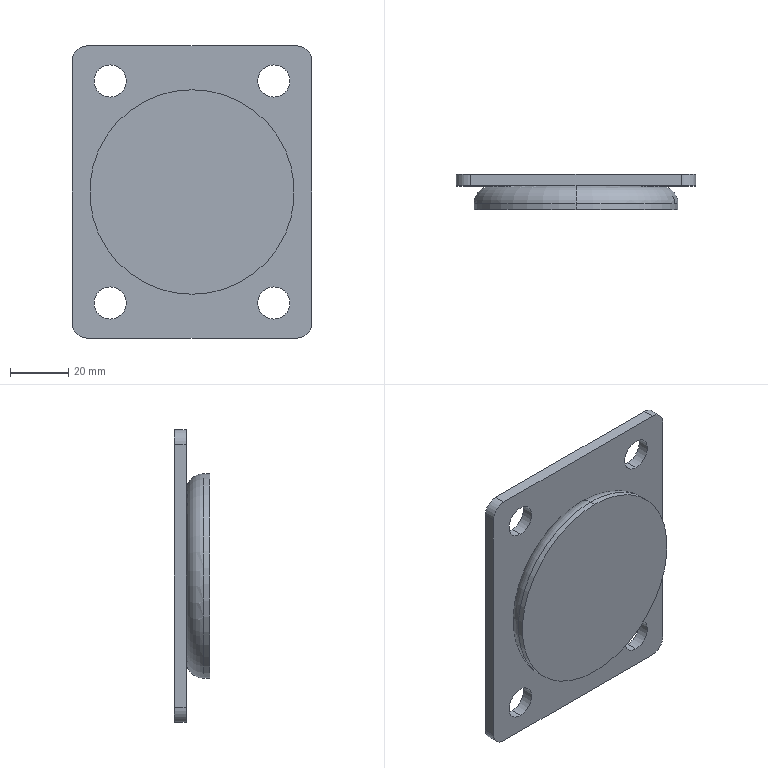Part | SolidWorks | features BaseBody 1 | 1 solid | 26 faces | box 82 x 12 x 100 mm | volume 48810 mm3 | cylinder 16 | plane 8 | torus 2 | commonest cylinder face diameters 11 x8 10 x4 70 x4
STEP:
#1=CARTESIAN_POINT('',(0.,60.5,21.));
#2=VERTEX_POINT('',#1);
#3=CARTESIAN_POINT('',(0.,60.5,-49.));
#4=VERTEX_POINT('',#3);
#5=CARTESIAN_POINT('',(0.,60.5,-14.));
#6=DIRECTION('',(0.,1.,0.));
#7=DIRECTION('',(0.,0.,1.));
#8=AXIS2_PLACEMENT_3D('',#5,#6,#7);
#9=CIRCLE('',#8,35.);
#10=EDGE_CURVE('',#2,#4,#9,.T.);
#11=ORIENTED_EDGE('',*,*,#10,.T.);
#12=CARTESIAN_POINT('',(0.,66.5,-43.));
#13=VERTEX_POINT('',#12);
#14=CARTESIAN_POINT('',(0.,60.5,-43.));
#15=DIRECTION('',(1.,0.,0.));
#16=DIRECTION('',(0.,0.,-1.));
#17=AXIS2_PLACEMENT_3D('',#14,#15,#16);
#18=CIRCLE('',#17,6.);
#19=EDGE_CURVE('',#4,#13,#18,.T.);
#20=ORIENTED_EDGE('',*,*,#19,.T.);
#21=CARTESIAN_POINT('',(0.,66.5,15.));
#22=VERTEX_POINT('',#21);
#23=CARTESIAN_POINT('',(0.,66.5,-43.));
#24=CARTESIAN_POINT('',(1.148,66.5,-43.));
#25=CARTESIAN_POINT('',(2.232,66.5,-42.932));
#26=CARTESIAN_POINT('',(4.262,66.5,-42.703));
#27=CARTESIAN_POINT('',(5.208,66.5,-42.542));
#28=CARTESIAN_POINT('',(7.832,66.5,-41.979));
#29=CARTESIAN_POINT('',(9.297,66.5,-41.499));
#30=CARTESIAN_POINT('',(11.688,66.5,-40.571));
#31=CARTESIAN_POINT('',(12.616,66.5,-40.124));
#32=CARTESIAN_POINT('',(13.391,66.5,-39.723));
#33=CARTESIAN_POINT('',(13.515,66.5,-39.659));
#34=CARTESIAN_POINT('',(13.635,66.5,-39.595));
#35=CARTESIAN_POINT('',(13.679,66.5,-39.571));
#36=CARTESIAN_POINT('',(13.686,66.5,-39.568));
#37=CARTESIAN_POINT('',(13.691,66.5,-39.565));
#38=CARTESIAN_POINT('',(13.699,66.5,-39.561));
#39=CARTESIAN_POINT('',(13.732,66.5,-39.543));
#40=CARTESIAN_POINT('',(13.81,66.5,-39.501));
#41=CARTESIAN_POINT('',(14.304,66.5,-39.232));
#42=CARTESIAN_POINT('',(14.766,66.5,-38.964));
#43=CARTESIAN_POINT('',(15.982,66.5,-38.218));
#44=CARTESIAN_POINT('',(16.772,66.5,-37.678));
#45=CARTESIAN_POINT('',(18.3,66.5,-36.518));
#46=CARTESIAN_POINT('',(19.038,66.5,-35.898));
#47=CARTESIAN_POINT('',(19.836,66.5,-35.156));
#48=CARTESIAN_POINT('',(19.924,66.5,-35.073));
#49=CARTESIAN_POINT('',(20.033,66.5,-34.969));
#50=CARTESIAN_POINT('',(20.056,66.5,-34.947));
#51=CARTESIAN_POINT('',(20.104,66.5,-34.901));
#52=CARTESIAN_POINT('',(20.175,66.5,-34.832));
#53=CARTESIAN_POINT('',(20.438,66.5,-34.577));
#54=CARTESIAN_POINT('',(21.047,66.5,-33.964));
#55=CARTESIAN_POINT('',(21.585,66.5,-33.374));
#56=CARTESIAN_POINT('',(22.63,66.5,-32.167));
#57=CARTESIAN_POINT('',(23.281,66.5,-31.324));
#58=CARTESIAN_POINT('',(24.036,66.5,-30.229));
#59=CARTESIAN_POINT('',(24.182,66.5,-30.011));
#60=CARTESIAN_POINT('',(24.481,66.5,-29.549));
#61=CARTESIAN_POINT('',(24.774,66.5,-29.084));
#62=CARTESIAN_POINT('',(25.123,66.5,-28.491));
#63=CARTESIAN_POINT('',(25.329,66.5,-28.124));
#64=CARTESIAN_POINT('',(25.399,66.5,-27.996));
#65=CARTESIAN_POINT('',(25.405,66.5,-27.985));
#66=CARTESIAN_POINT('',(25.408,66.5,-27.98));
#67=CARTESIAN_POINT('',(25.409,66.5,-27.978));
#68=CARTESIAN_POINT('',(25.411,66.5,-27.974));
#69=CARTESIAN_POINT('',(25.418,66.5,-27.962));
#70=CARTESIAN_POINT('',(25.435,66.5,-27.93));
#71=CARTESIAN_POINT('',(25.456,66.5,-27.892));
#72=CARTESIAN_POINT('',(25.538,66.5,-27.742));
#73=CARTESIAN_POINT('',(25.642,66.5,-27.549));
#74=CARTESIAN_POINT('',(25.92,66.5,-27.009));
#75=CARTESIAN_POINT('',(26.094,66.5,-26.663));
#76=CARTESIAN_POINT('',(26.342,66.5,-26.129));
#77=CARTESIAN_POINT('',(26.394,66.5,-26.017));
#78=CARTESIAN_POINT('',(26.453,66.5,-25.886));
#79=CARTESIAN_POINT('',(26.46,66.5,-25.871));
#80=CARTESIAN_POINT('',(26.469,66.5,-25.849));
#81=CARTESIAN_POINT('',(26.471,66.5,-25.846));
#82=CARTESIAN_POINT('',(26.474,66.5,-25.839));
#83=CARTESIAN_POINT('',(26.482,66.5,-25.821));
#84=CARTESIAN_POINT('',(26.503,66.5,-25.774));
#85=CARTESIAN_POINT('',(26.573,66.5,-25.615));
#86=CARTESIAN_POINT('',(26.638,66.5,-25.466));
#87=CARTESIAN_POINT('',(26.793,66.5,-25.101));
#88=CARTESIAN_POINT('',(26.897,66.5,-24.848));
#89=CARTESIAN_POINT('',(27.208,66.5,-24.054));
#90=CARTESIAN_POINT('',(27.415,66.5,-23.481));
#91=CARTESIAN_POINT('',(27.637,66.5,-22.788));
#92=CARTESIAN_POINT('',(27.674,66.5,-22.671));
#93=CARTESIAN_POINT('',(27.711,66.5,-22.553));
#94=CARTESIAN_POINT('',(27.726,66.5,-22.503));
#95=CARTESIAN_POINT('',(27.73,66.5,-22.49));
#96=CARTESIAN_POINT('',(27.731,66.5,-22.485));
#97=CARTESIAN_POINT('',(27.734,66.5,-22.477));
#98=CARTESIAN_POINT('',(27.75,66.5,-22.424));
#99=CARTESIAN_POINT('',(27.767,66.5,-22.367));
#100=CARTESIAN_POINT('',(27.817,66.5,-22.2));
#101=CARTESIAN_POINT('',(27.856,66.5,-22.068));
#102=CARTESIAN_POINT('',(27.987,66.5,-21.606));
#103=CARTESIAN_POINT('',(28.093,66.5,-21.214));
#104=CARTESIAN_POINT('',(28.322,66.5,-20.253));
#105=CARTESIAN_POINT('',(28.445,66.5,-19.685));
#106=CARTESIAN_POINT('',(28.677,66.5,-18.37));
#107=CARTESIAN_POINT('',(28.785,66.5,-17.622));
#108=CARTESIAN_POINT('',(28.906,66.5,-16.364));
#109=CARTESIAN_POINT('',(28.94,66.5,-15.923));
#110=CARTESIAN_POINT('',(28.975,66.5,-15.227));
#111=CARTESIAN_POINT('',(28.984,66.5,-14.989));
#112=CARTESIAN_POINT('',(28.994,66.5,-14.624));
#113=CARTESIAN_POINT('',(28.997,66.5,-14.44));
#114=CARTESIAN_POINT('',(28.999,66.5,-14.221));
#115=CARTESIAN_POINT('',(29.,66.5,-14.111));
#116=CARTESIAN_POINT('',(29.,66.5,-14.056));
#117=CARTESIAN_POINT('',(29.,66.5,-14.028));
#118=CARTESIAN_POINT('',(29.,66.5,-14.016));
#119=CARTESIAN_POINT('',(29.,66.5,-14.008));
#120=CARTESIAN_POINT('',(29.,66.5,-14.002));
#121=CARTESIAN_POINT('',(29.,66.5,-12.102));
#122=CARTESIAN_POINT('',(28.813,66.5,-10.204));
#123=CARTESIAN_POINT('',(28.073,66.5,-6.481));
#124=CARTESIAN_POINT('',(27.519,66.5,-4.656));
#125=CARTESIAN_POINT('',(26.066,66.5,-1.149));
#126=CARTESIAN_POINT('',(25.167,66.5,0.5335));
#127=CARTESIAN_POINT('',(23.058,66.5,3.69));
#128=CARTESIAN_POINT('',(21.848,66.5,5.164));
#129=CARTESIAN_POINT('',(19.164,66.5,7.848));
#130=CARTESIAN_POINT('',(17.69,66.5,9.058));
#131=CARTESIAN_POINT('',(14.533,66.5,11.167));
#132=CARTESIAN_POINT('',(12.851,66.5,12.066));
#133=CARTESIAN_POINT('',(9.344,66.5,13.519));
#134=CARTESIAN_POINT('',(7.519,66.5,14.073));
#135=CARTESIAN_POINT('',(3.796,66.5,14.813));
#136=CARTESIAN_POINT('',(1.898,66.5,15.));
#137=CARTESIAN_POINT('',(0.,66.5,15.));
#138=B_SPLINE_CURVE_WITH_KNOTS('',3,(#23,#24,#25,#26,#27,#28,#29,#30,#31,#32,#33,#34,#35,#36,#37,#38,#39,#40,#41,#42,#43,#44,#45,#46,#47,#48,#49,#50,#51,#52,#53,#54,#55,#56,#57,#58,#59,#60,#61,#62,#63,#64,#65,#66,#67,#68,#69,#70,#71,#72,#73,#74,#75,#76,#77,#78,#79,#80,#81,#82,#83,#84,#85,#86,#87,#88,#89,#90,#91,#92,#93,#94,#95,#96,#97,#98,#99,#100,#101,#102,#103,#104,#105,#106,#107,#108,#109,#110,#111,#112,#113,#114,#115,#116,#117,#118,#119,#120,#121,#122,#123,#124,#125,#126,#127,#128,#129,#130,#131,#132,#133,#134,#135,#136,#137),.UNSPECIFIED.,.F.,.F.,(4,2,2,2,2,1,1,1,2,2,1,1,2,2,2,2,2,1,1,1,2,2,2,1,1,1,2,2,1,1,1,2,2,2,2,2,2,1,1,1,2,2,2,1,2,2,1,1,2,2,2,2,2,2,2,1,1,1,1,1,2,2,2,2,2,2,2,2,2,4),(0.,0.03125,0.0625,0.125,0.1875,0.1953,0.1992,0.1997,0.2,0.2002,0.2012,0.2031,0.2188,0.25,0.2813,0.2852,0.2861,0.2871,0.2891,0.2969,0.3125,0.3438,0.3516,0.3594,0.3672,0.3711,0.3713,0.3715,0.3716,0.3721,0.373,0.375,0.3828,0.3906,0.3926,0.3928,0.3929,0.3931,0.3936,0.3945,0.3984,0.4063,0.4219,0.4238,0.4248,0.425,0.4253,0.4258,0.4297,0.4375,0.4531,0.4688,0.4844,0.4922,0.4961,0.498,0.499,0.4995,0.4998,0.4999,0.4999,0.5,0.5625,0.625,0.6875,0.75,0.8125,0.875,0.9375,1.),.UNSPECIFIED.);
#139=EDGE_CURVE('',#13,#22,#138,.T.);
#140=ORIENTED_EDGE('',*,*,#139,.T.);
#141=CARTESIAN_POINT('',(0.,60.5,15.));
#142=DIRECTION('',(-1.,0.,0.));
#143=DIRECTION('',(0.,0.,1.));
#144=AXIS2_PLACEMENT_3D('',#141,#142,#143);
#145=CIRCLE('',#144,6.);
#146=EDGE_CURVE('',#2,#22,#145,.T.);
#147=ORIENTED_EDGE('',*,*,#146,.F.);
#148=EDGE_LOOP('',(#11,#20,#140,#147));
#149=FACE_OUTER_BOUND('',#148,.T.);
#150=CARTESIAN_POINT('',(0.,60.5,-14.));
#151=DIRECTION('',(0.,1.,0.));
#152=DIRECTION('',(0.,0.,1.));
#153=AXIS2_PLACEMENT_3D('',#150,#151,#152);
#154=TOROIDAL_SURFACE('',#153,29.,6.);
#155=ADVANCED_FACE('',(#149),#154,.T.);
#156=CARTESIAN_POINT('',(-28.,66.5,-46.5));
#157=VERTEX_POINT('',#156);
#158=CARTESIAN_POINT('',(-28.,66.5,-57.5));
#159=VERTEX_POINT('',#158);
#160=CARTESIAN_POINT('',(-28.,66.5,-52.));
#161=DIRECTION('',(0.,-1.,0.));
#162=DIRECTION('',(0.,0.,1.));
#163=AXIS2_PLACEMENT_3D('',#160,#161,#162);
#164=CIRCLE('',#163,5.5);
#165=EDGE_CURVE('',#157,#159,#164,.T.);
#166=ORIENTED_EDGE('',*,*,#165,.T.);
#167=CARTESIAN_POINT('',(-28.,70.5,-57.5));
#168=VERTEX_POINT('',#167);
#169=CARTESIAN_POINT('',(-28.,58.5,-57.5));
#170=DIRECTION('',(0.,1.,0.));
#171=VECTOR('',#170,1000.);
#172=LINE('',#169,#171);
#173=EDGE_CURVE('',#159,#168,#172,.T.);
#174=ORIENTED_EDGE('',*,*,#173,.T.);
#175=CARTESIAN_POINT('',(-28.,70.5,-46.5));
#176=VERTEX_POINT('',#175);
#177=CARTESIAN_POINT('',(-28.,70.5,-52.));
#178=DIRECTION('',(0.,-1.,0.));
#179=DIRECTION('',(0.,0.,1.));
#180=AXIS2_PLACEMENT_3D('',#177,#178,#179);
#181=CIRCLE('',#180,5.5);
#182=EDGE_CURVE('',#176,#168,#181,.T.);
#183=ORIENTED_EDGE('',*,*,#182,.F.);
#184=CARTESIAN_POINT('',(-28.,58.5,-46.5));
#185=DIRECTION('',(0.,1.,0.));
#186=VECTOR('',#185,1000.);
#187=LINE('',#184,#186);
#188=EDGE_CURVE('',#157,#176,#187,.T.);
#189=ORIENTED_EDGE('',*,*,#188,.F.);
#190=EDGE_LOOP('',(#166,#174,#183,#189));
#191=FACE_OUTER_BOUND('',#190,.T.);
#192=CARTESIAN_POINT('',(-28.,58.5,-52.));
#193=DIRECTION('',(0.,1.,0.));
#194=DIRECTION('',(0.,0.,1.));
#195=AXIS2_PLACEMENT_3D('',#192,#193,#194);
#196=CYLINDRICAL_SURFACE('',#195,5.5);
#197=ADVANCED_FACE('',(#191),#196,.F.);
#198=CARTESIAN_POINT('',(28.,66.5,-46.5));
#199=VERTEX_POINT('',#198);
#200=CARTESIAN_POINT('',(28.,66.5,-57.5));
#201=VERTEX_POINT('',#200);
#202=CARTESIAN_POINT('',(28.,66.5,-52.));
#203=DIRECTION('',(0.,-1.,0.));
#204=DIRECTION('',(0.,0.,1.));
#205=AXIS2_PLACEMENT_3D('',#202,#203,#204);
#206=CIRCLE('',#205,5.5);
#207=EDGE_CURVE('',#199,#201,#206,.T.);
#208=ORIENTED_EDGE('',*,*,#207,.T.);
#209=CARTESIAN_POINT('',(28.,70.5,-57.5));
#210=VERTEX_POINT('',#209);
#211=CARTESIAN_POINT('',(28.,58.5,-57.5));
#212=DIRECTION('',(0.,1.,0.));
#213=VECTOR('',#212,1000.);
#214=LINE('',#211,#213);
#215=EDGE_CURVE('',#201,#210,#214,.T.);
#216=ORIENTED_EDGE('',*,*,#215,.T.);
#217=CARTESIAN_POINT('',(28.,70.5,-46.5));
#218=VERTEX_POINT('',#217);
#219=CARTESIAN_POINT('',(28.,70.5,-52.));
#220=DIRECTION('',(0.,-1.,0.));
#221=DIRECTION('',(0.,0.,1.));
#222=AXIS2_PLACEMENT_3D('',#219,#220,#221);
#223=CIRCLE('',#222,5.5);
#224=EDGE_CURVE('',#218,#210,#223,.T.);
#225=ORIENTED_EDGE('',*,*,#224,.F.);
#226=CARTESIAN_POINT('',(28.,58.5,-46.5));
#227=DIRECTION('',(0.,1.,0.));
#228=VECTOR('',#227,1000.);
#229=LINE('',#226,#228);
#230=EDGE_CURVE('',#199,#218,#229,.T.);
#231=ORIENTED_EDGE('',*,*,#230,.F.);
#232=EDGE_LOOP('',(#208,#216,#225,#231));
#233=FACE_OUTER_BOUND('',#232,.T.);
#234=CARTESIAN_POINT('',(28.,58.5,-52.));
#235=DIRECTION('',(0.,1.,0.));
#236=DIRECTION('',(0.,0.,1.));
#237=AXIS2_PLACEMENT_3D('',#234,#235,#236);
#238=CYLINDRICAL_SURFACE('',#237,5.5);
#239=ADVANCED_FACE('',(#233),#238,.F.);
#240=CARTESIAN_POINT('',(28.,66.5,29.5));
#241=VERTEX_POINT('',#240);
#242=CARTESIAN_POINT('',(28.,66.5,18.5));
#243=VERTEX_POINT('',#242);
#244=CARTESIAN_POINT('',(28.,66.5,24.));
#245=DIRECTION('',(0.,-1.,0.));
#246=DIRECTION('',(0.,0.,1.));
#247=AXIS2_PLACEMENT_3D('',#244,#245,#246);
#248=CIRCLE('',#247,5.5);
#249=EDGE_CURVE('',#241,#243,#248,.T.);
#250=ORIENTED_EDGE('',*,*,#249,.T.);
#251=CARTESIAN_POINT('',(28.,70.5,18.5));
#252=VERTEX_POINT('',#251);
#253=CARTESIAN_POINT('',(28.,58.5,18.5));
#254=DIRECTION('',(0.,1.,0.));
#255=VECTOR('',#254,1000.);
#256=LINE('',#253,#255);
#257=EDGE_CURVE('',#243,#252,#256,.T.);
#258=ORIENTED_EDGE('',*,*,#257,.T.);
#259=CARTESIAN_POINT('',(28.,70.5,29.5));
#260=VERTEX_POINT('',#259);
#261=CARTESIAN_POINT('',(28.,70.5,24.));
#262=DIRECTION('',(0.,-1.,0.));
#263=DIRECTION('',(0.,0.,1.));
#264=AXIS2_PLACEMENT_3D('',#261,#262,#263);
#265=CIRCLE('',#264,5.5);
#266=EDGE_CURVE('',#260,#252,#265,.T.);
#267=ORIENTED_EDGE('',*,*,#266,.F.);
#268=CARTESIAN_POINT('',(28.,58.5,29.5));
#269=DIRECTION('',(0.,1.,0.));
#270=VECTOR('',#269,1000.);
#271=LINE('',#268,#270);
#272=EDGE_CURVE('',#241,#260,#271,.T.);
#273=ORIENTED_EDGE('',*,*,#272,.F.);
#274=EDGE_LOOP('',(#250,#258,#267,#273));
#275=FACE_OUTER_BOUND('',#274,.T.);
#276=CARTESIAN_POINT('',(28.,58.5,24.));
#277=DIRECTION('',(0.,1.,0.));
#278=DIRECTION('',(0.,0.,1.));
#279=AXIS2_PLACEMENT_3D('',#276,#277,#278);
#280=CYLINDRICAL_SURFACE('',#279,5.5);
#281=ADVANCED_FACE('',(#275),#280,.F.);
#282=CARTESIAN_POINT('',(-28.,66.5,29.5));
#283=VERTEX_POINT('',#282);
#284=CARTESIAN_POINT('',(-28.,66.5,18.5));
#285=VERTEX_POINT('',#284);
#286=CARTESIAN_POINT('',(-28.,66.5,24.));
#287=DIRECTION('',(0.,-1.,0.));
#288=DIRECTION('',(0.,0.,1.));
#289=AXIS2_PLACEMENT_3D('',#286,#287,#288);
#290=CIRCLE('',#289,5.5);
#291=EDGE_CURVE('',#283,#285,#290,.T.);
#292=ORIENTED_EDGE('',*,*,#291,.T.);
#293=CARTESIAN_POINT('',(-28.,70.5,18.5));
#294=VERTEX_POINT('',#293);
#295=CARTESIAN_POINT('',(-28.,58.5,18.5));
#296=DIRECTION('',(0.,1.,0.));
#297=VECTOR('',#296,1000.);
#298=LINE('',#295,#297);
#299=EDGE_CURVE('',#285,#294,#298,.T.);
#300=ORIENTED_EDGE('',*,*,#299,.T.);
#301=CARTESIAN_POINT('',(-28.,70.5,29.5));
#302=VERTEX_POINT('',#301);
#303=CARTESIAN_POINT('',(-28.,70.5,24.));
#304=DIRECTION('',(0.,-1.,0.));
#305=DIRECTION('',(0.,0.,1.));
#306=AXIS2_PLACEMENT_3D('',#303,#304,#305);
#307=CIRCLE('',#306,5.5);
#308=EDGE_CURVE('',#302,#294,#307,.T.);
#309=ORIENTED_EDGE('',*,*,#308,.F.);
#310=CARTESIAN_POINT('',(-28.,58.5,29.5));
#311=DIRECTION('',(0.,1.,0.));
#312=VECTOR('',#311,1000.);
#313=LINE('',#310,#312);
#314=EDGE_CURVE('',#283,#302,#313,.T.);
#315=ORIENTED_EDGE('',*,*,#314,.F.);
#316=EDGE_LOOP('',(#292,#300,#309,#315));
#317=FACE_OUTER_BOUND('',#316,.T.);
#318=CARTESIAN_POINT('',(-28.,58.5,24.));
#319=DIRECTION('',(0.,1.,0.));
#320=DIRECTION('',(0.,0.,1.));
#321=AXIS2_PLACEMENT_3D('',#318,#319,#320);
#322=CYLINDRICAL_SURFACE('',#321,5.5);
#323=ADVANCED_FACE('',(#317),#322,.F.);
#324=ORIENTED_EDGE('',*,*,#10,.F.);
#325=CARTESIAN_POINT('',(0.,58.5,21.));
#326=VERTEX_POINT('',#325);
#327=CARTESIAN_POINT('',(0.,500.,21.));
#328=DIRECTION('',(0.,-1.,0.));
#329=VECTOR('',#328,1000.);
#330=LINE('',#327,#329);
#331=EDGE_CURVE('',#2,#326,#330,.T.);
#332=ORIENTED_EDGE('',*,*,#331,.T.);
#333=CARTESIAN_POINT('',(0.,58.5,-49.));
#334=VERTEX_POINT('',#333);
#335=CARTESIAN_POINT('',(0.,58.5,-14.));
#336=DIRECTION('',(0.,1.,0.));
#337=DIRECTION('',(0.,0.,-1.));
#338=AXIS2_PLACEMENT_3D('',#335,#336,#337);
#339=CIRCLE('',#338,35.);
#340=EDGE_CURVE('',#326,#334,#339,.T.);
#341=ORIENTED_EDGE('',*,*,#340,.T.);
#342=CARTESIAN_POINT('',(0.,500.,-49.));
#343=DIRECTION('',(0.,-1.,0.));
#344=VECTOR('',#343,1000.);
#345=LINE('',#342,#344);
#346=EDGE_CURVE('',#4,#334,#345,.T.);
#347=ORIENTED_EDGE('',*,*,#346,.F.);
#348=EDGE_LOOP('',(#324,#332,#341,#347));
#349=FACE_OUTER_BOUND('',#348,.T.);
#350=CARTESIAN_POINT('',(0.,500.,-14.));
#351=DIRECTION('',(0.,-1.,0.));
#352=DIRECTION('',(0.,0.,-1.));
#353=AXIS2_PLACEMENT_3D('',#350,#351,#352);
#354=CYLINDRICAL_SURFACE('',#353,35.);
#355=ADVANCED_FACE('',(#349),#354,.T.);
#356=CARTESIAN_POINT('',(0.,70.5,21.));
#357=VERTEX_POINT('',#356);
#358=CARTESIAN_POINT('',(0.,70.5,-49.));
#359=VERTEX_POINT('',#358);
#360=CARTESIAN_POINT('',(0.,70.5,-14.));
#361=DIRECTION('',(0.,-1.,0.));
#362=DIRECTION('',(0.,0.,-1.));
#363=AXIS2_PLACEMENT_3D('',#360,#361,#362);
#364=CIRCLE('',#363,35.);
#365=EDGE_CURVE('',#357,#359,#364,.T.);
#366=ORIENTED_EDGE('',*,*,#365,.F.);
#367=CARTESIAN_POINT('',(0.,67.5,21.));
#368=VERTEX_POINT('',#367);
#369=CARTESIAN_POINT('',(0.,67.5,21.));
#370=DIRECTION('',(0.,-1.,0.));
#371=VECTOR('',#370,1000.);
#372=LINE('',#369,#371);
#373=EDGE_CURVE('',#357,#368,#372,.T.);
#374=ORIENTED_EDGE('',*,*,#373,.T.);
#375=CARTESIAN_POINT('',(0.,67.5,-49.));
#376=VERTEX_POINT('',#375);
#377=CARTESIAN_POINT('',(0.,67.5,-14.));
#378=DIRECTION('',(0.,1.,0.));
#379=DIRECTION('',(0.,0.,-1.));
#380=AXIS2_PLACEMENT_3D('',#377,#378,#379);
#381=CIRCLE('',#380,35.);
#382=EDGE_CURVE('',#376,#368,#381,.T.);
#383=ORIENTED_EDGE('',*,*,#382,.F.);
#384=CARTESIAN_POINT('',(0.,67.5,-49.));
#385=DIRECTION('',(0.,-1.,0.));
#386=VECTOR('',#385,1000.);
#387=LINE('',#384,#386);
#388=EDGE_CURVE('',#359,#376,#387,.T.);
#389=ORIENTED_EDGE('',*,*,#388,.F.);
#390=EDGE_LOOP('',(#366,#374,#383,#389));
#391=FACE_OUTER_BOUND('',#390,.T.);
#392=CARTESIAN_POINT('',(0.,67.5,-14.));
#393=DIRECTION('',(0.,-1.,0.));
#394=DIRECTION('',(0.,0.,-1.));
#395=AXIS2_PLACEMENT_3D('',#392,#393,#394);
#396=CYLINDRICAL_SURFACE('',#395,35.);
#397=ADVANCED_FACE('',(#391),#396,.F.);
#398=ORIENTED_EDGE('',*,*,#139,.F.);
#399=CARTESIAN_POINT('',(0.,66.5,15.));
#400=CARTESIAN_POINT('',(-1.148,66.5,15.));
#401=CARTESIAN_POINT('',(-2.232,66.5,14.932));
#402=CARTESIAN_POINT('',(-4.262,66.5,14.703));
#403=CARTESIAN_POINT('',(-5.208,66.5,14.542));
#404=CARTESIAN_POINT('',(-7.832,66.5,13.979));
#405=CARTESIAN_POINT('',(-9.296,66.5,13.499));
#406=CARTESIAN_POINT('',(-11.687,66.5,12.571));
#407=CARTESIAN_POINT('',(-12.616,66.5,12.124));
#408=CARTESIAN_POINT('',(-13.391,66.5,11.723));
#409=CARTESIAN_POINT('',(-13.515,66.5,11.659));
#410=CARTESIAN_POINT('',(-13.635,66.5,11.595));
#411=CARTESIAN_POINT('',(-13.679,66.5,11.571));
#412=CARTESIAN_POINT('',(-13.686,66.5,11.568));
#413=CARTESIAN_POINT('',(-13.691,66.5,11.565));
#414=CARTESIAN_POINT('',(-13.699,66.5,11.561));
#415=CARTESIAN_POINT('',(-13.732,66.5,11.543));
#416=CARTESIAN_POINT('',(-13.81,66.5,11.501));
#417=CARTESIAN_POINT('',(-14.304,66.5,11.232));
#418=CARTESIAN_POINT('',(-14.766,66.5,10.964));
#419=CARTESIAN_POINT('',(-15.982,66.5,10.218));
#420=CARTESIAN_POINT('',(-16.772,66.5,9.678));
#421=CARTESIAN_POINT('',(-18.3,66.5,8.518));
#422=CARTESIAN_POINT('',(-19.038,66.5,7.898));
#423=CARTESIAN_POINT('',(-19.836,66.5,7.156));
#424=CARTESIAN_POINT('',(-19.924,66.5,7.073));
#425=CARTESIAN_POINT('',(-20.033,66.5,6.969));
#426=CARTESIAN_POINT('',(-20.056,66.5,6.947));
#427=CARTESIAN_POINT('',(-20.104,66.5,6.901));
#428=CARTESIAN_POINT('',(-20.175,66.5,6.832));
#429=CARTESIAN_POINT('',(-20.438,66.5,6.577));
#430=CARTESIAN_POINT('',(-21.047,66.5,5.964));
#431=CARTESIAN_POINT('',(-21.585,66.5,5.374));
#432=CARTESIAN_POINT('',(-22.63,66.5,4.167));
#433=CARTESIAN_POINT('',(-23.281,66.5,3.324));
#434=CARTESIAN_POINT('',(-24.036,66.5,2.229));
#435=CARTESIAN_POINT('',(-24.182,66.5,2.011));
#436=CARTESIAN_POINT('',(-24.481,66.5,1.549));
#437=CARTESIAN_POINT('',(-24.774,66.5,1.084));
#438=CARTESIAN_POINT('',(-25.123,66.5,0.4912));
#439=CARTESIAN_POINT('',(-25.329,66.5,0.1238));
#440=CARTESIAN_POINT('',(-25.399,66.5,-0.004153));
#441=CARTESIAN_POINT('',(-25.405,66.5,-0.01545));
#442=CARTESIAN_POINT('',(-25.408,66.5,-0.01988));
#443=CARTESIAN_POINT('',(-25.409,66.5,-0.02154));
#444=CARTESIAN_POINT('',(-25.411,66.5,-0.02578));
#445=CARTESIAN_POINT('',(-25.418,66.5,-0.03795));
#446=CARTESIAN_POINT('',(-25.435,66.5,-0.07019));
#447=CARTESIAN_POINT('',(-25.456,66.5,-0.1082));
#448=CARTESIAN_POINT('',(-25.538,66.5,-0.2579));
#449=CARTESIAN_POINT('',(-25.642,66.5,-0.4514));
#450=CARTESIAN_POINT('',(-25.92,66.5,-0.9911));
#451=CARTESIAN_POINT('',(-26.094,66.5,-1.337));
#452=CARTESIAN_POINT('',(-26.342,66.5,-1.871));
#453=CARTESIAN_POINT('',(-26.394,66.5,-1.983));
#454=CARTESIAN_POINT('',(-26.453,66.5,-2.114));
#455=CARTESIAN_POINT('',(-26.46,66.5,-2.129));
#456=CARTESIAN_POINT('',(-26.469,66.5,-2.151));
#457=CARTESIAN_POINT('',(-26.471,66.5,-2.154));
#458=CARTESIAN_POINT('',(-26.474,66.5,-2.161));
#459=CARTESIAN_POINT('',(-26.482,66.5,-2.179));
#460=CARTESIAN_POINT('',(-26.503,66.5,-2.226));
#461=CARTESIAN_POINT('',(-26.573,66.5,-2.385));
#462=CARTESIAN_POINT('',(-26.638,66.5,-2.534));
#463=CARTESIAN_POINT('',(-26.793,66.5,-2.899));
#464=CARTESIAN_POINT('',(-26.897,66.5,-3.152));
#465=CARTESIAN_POINT('',(-27.208,66.5,-3.946));
#466=CARTESIAN_POINT('',(-27.415,66.5,-4.519));
#467=CARTESIAN_POINT('',(-27.637,66.5,-5.212));
#468=CARTESIAN_POINT('',(-27.674,66.5,-5.329));
#469=CARTESIAN_POINT('',(-27.711,66.5,-5.447));
#470=CARTESIAN_POINT('',(-27.726,66.5,-5.497));
#471=CARTESIAN_POINT('',(-27.73,66.5,-5.51));
#472=CARTESIAN_POINT('',(-27.731,66.5,-5.515));
#473=CARTESIAN_POINT('',(-27.734,66.5,-5.523));
#474=CARTESIAN_POINT('',(-27.75,66.5,-5.576));
#475=CARTESIAN_POINT('',(-27.767,66.5,-5.633));
#476=CARTESIAN_POINT('',(-27.817,66.5,-5.8));
#477=CARTESIAN_POINT('',(-27.856,66.5,-5.932));
#478=CARTESIAN_POINT('',(-27.987,66.5,-6.394));
#479=CARTESIAN_POINT('',(-28.093,66.5,-6.786));
#480=CARTESIAN_POINT('',(-28.322,66.5,-7.747));
#481=CARTESIAN_POINT('',(-28.445,66.5,-8.315));
#482=CARTESIAN_POINT('',(-28.677,66.5,-9.63));
#483=CARTESIAN_POINT('',(-28.785,66.5,-10.378));
#484=CARTESIAN_POINT('',(-28.906,66.5,-11.636));
#485=CARTESIAN_POINT('',(-28.94,66.5,-12.077));
#486=CARTESIAN_POINT('',(-28.975,66.5,-12.773));
#487=CARTESIAN_POINT('',(-28.984,66.5,-13.011));
#488=CARTESIAN_POINT('',(-28.994,66.5,-13.376));
#489=CARTESIAN_POINT('',(-28.997,66.5,-13.56));
#490=CARTESIAN_POINT('',(-28.999,66.5,-13.779));
#491=CARTESIAN_POINT('',(-29.,66.5,-13.889));
#492=CARTESIAN_POINT('',(-29.,66.5,-13.944));
#493=CARTESIAN_POINT('',(-29.,66.5,-13.972));
#494=CARTESIAN_POINT('',(-29.,66.5,-13.984));
#495=CARTESIAN_POINT('',(-29.,66.5,-13.992));
#496=CARTESIAN_POINT('',(-29.,66.5,-13.998));
#497=CARTESIAN_POINT('',(-29.,66.5,-15.898));
#498=CARTESIAN_POINT('',(-28.813,66.5,-17.796));
#499=CARTESIAN_POINT('',(-28.073,66.5,-21.519));
#500=CARTESIAN_POINT('',(-27.519,66.5,-23.344));
#501=CARTESIAN_POINT('',(-26.066,66.5,-26.851));
#502=CARTESIAN_POINT('',(-25.167,66.5,-28.533));
#503=CARTESIAN_POINT('',(-23.058,66.5,-31.69));
#504=CARTESIAN_POINT('',(-21.848,66.5,-33.164));
#505=CARTESIAN_POINT('',(-19.164,66.5,-35.848));
#506=CARTESIAN_POINT('',(-17.69,66.5,-37.058));
#507=CARTESIAN_POINT('',(-14.533,66.5,-39.167));
#508=CARTESIAN_POINT('',(-12.851,66.5,-40.066));
#509=CARTESIAN_POINT('',(-9.344,66.5,-41.519));
#510=CARTESIAN_POINT('',(-7.519,66.5,-42.073));
#511=CARTESIAN_POINT('',(-3.796,66.5,-42.813));
#512=CARTESIAN_POINT('',(-1.898,66.5,-43.));
#513=CARTESIAN_POINT('',(0.,66.5,-43.));
#514=B_SPLINE_CURVE_WITH_KNOTS('',3,(#399,#400,#401,#402,#403,#404,#405,#406,#407,#408,#409,#410,#411,#412,#413,#414,#415,#416,#417,#418,#419,#420,#421,#422,#423,#424,#425,#426,#427,#428,#429,#430,#431,#432,#433,#434,#435,#436,#437,#438,#439,#440,#441,#442,#443,#444,#445,#446,#447,#448,#449,#450,#451,#452,#453,#454,#455,#456,#457,#458,#459,#460,#461,#462,#463,#464,#465,#466,#467,#468,#469,#470,#471,#472,#473,#474,#475,#476,#477,#478,#479,#480,#481,#482,#483,#484,#485,#486,#487,#488,#489,#490,#491,#492,#493,#494,#495,#496,#497,#498,#499,#500,#501,#502,#503,#504,#505,#506,#507,#508,#509,#510,#511,#512,#513),.UNSPECIFIED.,.F.,.F.,(4,2,2,2,2,1,1,1,2,2,1,1,2,2,2,2,2,1,1,1,2,2,2,1,1,1,2,2,1,1,1,2,2,2,2,2,2,1,1,1,2,2,2,1,2,2,1,1,2,2,2,2,2,2,2,1,1,1,1,1,2,2,2,2,2,2,2,2,2,4),(0.,0.03125,0.0625,0.125,0.1875,0.1953,0.1992,0.1997,0.2,0.2002,0.2012,0.2031,0.2188,0.25,0.2813,0.2852,0.2861,0.2871,0.2891,0.2969,0.3125,0.3438,0.3516,0.3594,0.3672,0.3711,0.3713,0.3715,0.3716,0.3721,0.373,0.375,0.3828,0.3906,0.3926,0.3928,0.3929,0.3931,0.3936,0.3945,0.3984,0.4063,0.4219,0.4238,0.4248,0.425,0.4253,0.4258,0.4297,0.4375,0.4531,0.4688,0.4844,0.4922,0.4961,0.498,0.499,0.4995,0.4998,0.4999,0.4999,0.5,0.5625,0.625,0.6875,0.75,0.8125,0.875,0.9375,1.),.UNSPECIFIED.);
#515=EDGE_CURVE('',#22,#13,#514,.T.);
#516=ORIENTED_EDGE('',*,*,#515,.F.);
#517=EDGE_LOOP('',(#398,#516));
#518=FACE_BOUND('',#517,.T.);
#519=CARTESIAN_POINT('',(-36.,66.5,-64.));
#520=VERTEX_POINT('',#519);
#521=CARTESIAN_POINT('',(-41.,66.5,-59.));
#522=VERTEX_POINT('',#521);
#523=CARTESIAN_POINT('',(-36.,66.5,-59.));
#524=DIRECTION('',(0.,1.,0.));
#525=DIRECTION('',(0.,0.,1.));
#526=AXIS2_PLACEMENT_3D('',#523,#524,#525);
#527=CIRCLE('',#526,5.);
#528=EDGE_CURVE('',#520,#522,#527,.T.);
#529=ORIENTED_EDGE('',*,*,#528,.F.);
#530=CARTESIAN_POINT('',(36.,66.5,-64.));
#531=VERTEX_POINT('',#530);
#532=CARTESIAN_POINT('',(-42.,66.5,-64.));
#533=DIRECTION('',(-1.,0.,0.));
#534=VECTOR('',#533,1000.);
#535=LINE('',#532,#534);
#536=EDGE_CURVE('',#531,#520,#535,.T.);
#537=ORIENTED_EDGE('',*,*,#536,.F.);
#538=CARTESIAN_POINT('',(41.,66.5,-59.));
#539=VERTEX_POINT('',#538);
#540=CARTESIAN_POINT('',(36.,66.5,-59.));
#541=DIRECTION('',(0.,1.,0.));
#542=DIRECTION('',(0.,0.,-1.));
#543=AXIS2_PLACEMENT_3D('',#540,#541,#542);
#544=CIRCLE('',#543,5.);
#545=EDGE_CURVE('',#539,#531,#544,.T.);
#546=ORIENTED_EDGE('',*,*,#545,.F.);
#547=CARTESIAN_POINT('',(41.,66.5,31.));
#548=VERTEX_POINT('',#547);
#549=CARTESIAN_POINT('',(41.,66.5,28.));
#550=DIRECTION('',(0.,0.,-1.));
#551=VECTOR('',#550,1000.);
#552=LINE('',#549,#551);
#553=EDGE_CURVE('',#548,#539,#552,.T.);
#554=ORIENTED_EDGE('',*,*,#553,.F.);
#555=CARTESIAN_POINT('',(36.,66.5,36.));
#556=VERTEX_POINT('',#555);
#557=CARTESIAN_POINT('',(36.,66.5,31.));
#558=DIRECTION('',(0.,1.,0.));
#559=DIRECTION('',(0.,0.,1.));
#560=AXIS2_PLACEMENT_3D('',#557,#558,#559);
#561=CIRCLE('',#560,5.);
#562=EDGE_CURVE('',#556,#548,#561,.T.);
#563=ORIENTED_EDGE('',*,*,#562,.F.);
#564=CARTESIAN_POINT('',(-36.,66.5,36.));
#565=VERTEX_POINT('',#564);
#566=CARTESIAN_POINT('',(-42.,66.5,36.));
#567=DIRECTION('',(1.,0.,0.));
#568=VECTOR('',#567,1000.);
#569=LINE('',#566,#568);
#570=EDGE_CURVE('',#565,#556,#569,.T.);
#571=ORIENTED_EDGE('',*,*,#570,.F.);
#572=CARTESIAN_POINT('',(-41.,66.5,31.));
#573=VERTEX_POINT('',#572);
#574=CARTESIAN_POINT('',(-36.,66.5,31.));
#575=DIRECTION('',(0.,1.,0.));
#576=DIRECTION('',(0.,0.,-1.));
#577=AXIS2_PLACEMENT_3D('',#574,#575,#576);
#578=CIRCLE('',#577,5.);
#579=EDGE_CURVE('',#573,#565,#578,.T.);
#580=ORIENTED_EDGE('',*,*,#579,.F.);
#581=CARTESIAN_POINT('',(-41.,66.5,28.));
#582=DIRECTION('',(0.,0.,1.));
#583=VECTOR('',#582,1000.);
#584=LINE('',#581,#583);
#585=EDGE_CURVE('',#522,#573,#584,.T.);
#586=ORIENTED_EDGE('',*,*,#585,.F.);
#587=EDGE_LOOP('',(#529,#537,#546,#554,#563,#571,#580,#586));
#588=FACE_OUTER_BOUND('',#587,.T.);
#589=ORIENTED_EDGE('',*,*,#165,.F.);
#590=CARTESIAN_POINT('',(-28.,66.5,-52.));
#591=DIRECTION('',(0.,-1.,0.));
#592=DIRECTION('',(0.,0.,1.));
#593=AXIS2_PLACEMENT_3D('',#590,#591,#592);
#594=CIRCLE('',#593,5.5);
#595=EDGE_CURVE('',#159,#157,#594,.T.);
#596=ORIENTED_EDGE('',*,*,#595,.F.);
#597=EDGE_LOOP('',(#589,#596));
#598=FACE_BOUND('',#597,.T.);
#599=ORIENTED_EDGE('',*,*,#207,.F.);
#600=CARTESIAN_POINT('',(28.,66.5,-52.));
#601=DIRECTION('',(0.,-1.,0.));
#602=DIRECTION('',(0.,0.,1.));
#603=AXIS2_PLACEMENT_3D('',#600,#601,#602);
#604=CIRCLE('',#603,5.5);
#605=EDGE_CURVE('',#201,#199,#604,.T.);
#606=ORIENTED_EDGE('',*,*,#605,.F.);
#607=EDGE_LOOP('',(#599,#606));
#608=FACE_BOUND('',#607,.T.);
#609=ORIENTED_EDGE('',*,*,#249,.F.);
#610=CARTESIAN_POINT('',(28.,66.5,24.));
#611=DIRECTION('',(0.,-1.,0.));
#612=DIRECTION('',(0.,0.,1.));
#613=AXIS2_PLACEMENT_3D('',#610,#611,#612);
#614=CIRCLE('',#613,5.5);
#615=EDGE_CURVE('',#243,#241,#614,.T.);
#616=ORIENTED_EDGE('',*,*,#615,.F.);
#617=EDGE_LOOP('',(#609,#616));
#618=FACE_BOUND('',#617,.T.);
#619=ORIENTED_EDGE('',*,*,#291,.F.);
#620=CARTESIAN_POINT('',(-28.,66.5,24.));
#621=DIRECTION('',(0.,-1.,0.));
#622=DIRECTION('',(0.,0.,1.));
#623=AXIS2_PLACEMENT_3D('',#620,#621,#622);
#624=CIRCLE('',#623,5.5);
#625=EDGE_CURVE('',#285,#283,#624,.T.);
#626=ORIENTED_EDGE('',*,*,#625,.F.);
#627=EDGE_LOOP('',(#619,#626));
#628=FACE_BOUND('',#627,.T.);
#629=CARTESIAN_POINT('',(-42.,66.5,28.));
#630=DIRECTION('',(0.,1.,0.));
#631=DIRECTION('',(0.,0.,1.));
#632=AXIS2_PLACEMENT_3D('',#629,#630,#631);
#633=PLANE('',#632);
#634=ADVANCED_FACE('',(#518,#588,#598,#608,#618,#628),#633,.F.);
#635=ORIENTED_EDGE('',*,*,#19,.F.);
#636=CARTESIAN_POINT('',(0.,60.5,-14.));
#637=DIRECTION('',(0.,1.,0.));
#638=DIRECTION('',(0.,0.,1.));
#639=AXIS2_PLACEMENT_3D('',#636,#637,#638);
#640=CIRCLE('',#639,35.);
#641=EDGE_CURVE('',#4,#2,#640,.T.);
#642=ORIENTED_EDGE('',*,*,#641,.T.);
#643=ORIENTED_EDGE('',*,*,#146,.T.);
#644=ORIENTED_EDGE('',*,*,#515,.T.);
#645=EDGE_LOOP('',(#635,#642,#643,#644));
#646=FACE_OUTER_BOUND('',#645,.T.);
#647=CARTESIAN_POINT('',(0.,60.5,-14.));
#648=DIRECTION('',(0.,1.,0.));
#649=DIRECTION('',(0.,0.,1.));
#650=AXIS2_PLACEMENT_3D('',#647,#648,#649);
#651=TOROIDAL_SURFACE('',#650,29.,6.);
#652=ADVANCED_FACE('',(#646),#651,.T.);
#653=CARTESIAN_POINT('',(-41.,70.5,-59.));
#654=VERTEX_POINT('',#653);
#655=CARTESIAN_POINT('',(-41.,58.5,-59.));
#656=DIRECTION('',(0.,1.,0.));
#657=VECTOR('',#656,1000.);
#658=LINE('',#655,#657);
#659=EDGE_CURVE('',#522,#654,#658,.T.);
#660=ORIENTED_EDGE('',*,*,#659,.F.);
#661=ORIENTED_EDGE('',*,*,#585,.T.);
#662=CARTESIAN_POINT('',(-41.,70.5,31.));
#663=VERTEX_POINT('',#662);
#664=CARTESIAN_POINT('',(-41.,58.5,31.));
#665=DIRECTION('',(0.,-1.,0.));
#666=VECTOR('',#665,1000.);
#667=LINE('',#664,#666);
#668=EDGE_CURVE('',#663,#573,#667,.T.);
#669=ORIENTED_EDGE('',*,*,#668,.F.);
#670=CARTESIAN_POINT('',(-41.,70.5,-74.509));
#671=DIRECTION('',(0.,0.,1.));
#672=VECTOR('',#671,1000.);
#673=LINE('',#670,#672);
#674=EDGE_CURVE('',#654,#663,#673,.T.);
#675=ORIENTED_EDGE('',*,*,#674,.F.);
#676=EDGE_LOOP('',(#660,#661,#669,#675));
#677=FACE_OUTER_BOUND('',#676,.T.);
#678=CARTESIAN_POINT('',(-41.,58.5,-74.509));
#679=DIRECTION('',(1.,0.,0.));
#680=DIRECTION('',(0.,0.,-1.));
#681=AXIS2_PLACEMENT_3D('',#678,#679,#680);
#682=PLANE('',#681);
#683=ADVANCED_FACE('',(#677),#682,.F.);
#684=ORIENTED_EDGE('',*,*,#528,.T.);
#685=ORIENTED_EDGE('',*,*,#659,.T.);
#686=CARTESIAN_POINT('',(-36.,70.5,-64.));
#687=VERTEX_POINT('',#686);
#688=CARTESIAN_POINT('',(-36.,70.5,-59.));
#689=DIRECTION('',(0.,-1.,0.));
#690=DIRECTION('',(0.,0.,1.));
#691=AXIS2_PLACEMENT_3D('',#688,#689,#690);
#692=CIRCLE('',#691,5.);
#693=EDGE_CURVE('',#654,#687,#692,.T.);
#694=ORIENTED_EDGE('',*,*,#693,.T.);
#695=CARTESIAN_POINT('',(-36.,58.5,-64.));
#696=DIRECTION('',(0.,-1.,0.));
#697=VECTOR('',#696,1000.);
#698=LINE('',#695,#697);
#699=EDGE_CURVE('',#687,#520,#698,.T.);
#700=ORIENTED_EDGE('',*,*,#699,.T.);
#701=EDGE_LOOP('',(#684,#685,#694,#700));
#702=FACE_OUTER_BOUND('',#701,.T.);
#703=CARTESIAN_POINT('',(-36.,58.5,-59.));
#704=DIRECTION('',(0.,1.,0.));
#705=DIRECTION('',(0.,0.,1.));
#706=AXIS2_PLACEMENT_3D('',#703,#704,#705);
#707=CYLINDRICAL_SURFACE('',#706,5.);
#708=ADVANCED_FACE('',(#702),#707,.T.);
#709=CARTESIAN_POINT('',(36.,70.5,-64.));
#710=VERTEX_POINT('',#709);
#711=CARTESIAN_POINT('',(42.,70.5,-64.));
#712=DIRECTION('',(1.,0.,0.));
#713=VECTOR('',#712,1000.);
#714=LINE('',#711,#713);
#715=EDGE_CURVE('',#687,#710,#714,.T.);
#716=ORIENTED_EDGE('',*,*,#715,.T.);
#717=CARTESIAN_POINT('',(36.,66.5,-64.));
#718=DIRECTION('',(0.,-1.,0.));
#719=VECTOR('',#718,1000.);
#720=LINE('',#717,#719);
#721=EDGE_CURVE('',#710,#531,#720,.T.);
#722=ORIENTED_EDGE('',*,*,#721,.T.);
#723=ORIENTED_EDGE('',*,*,#536,.T.);
#724=ORIENTED_EDGE('',*,*,#699,.F.);
#725=EDGE_LOOP('',(#716,#722,#723,#724));
#726=FACE_OUTER_BOUND('',#725,.T.);
#727=CARTESIAN_POINT('',(42.,66.5,-64.));
#728=DIRECTION('',(0.,0.,-1.));
#729=DIRECTION('',(-1.,0.,0.));
#730=AXIS2_PLACEMENT_3D('',#727,#728,#729);
#731=PLANE('',#730);
#732=ADVANCED_FACE('',(#726),#731,.T.);
#733=CARTESIAN_POINT('',(41.,70.5,-59.));
#734=VERTEX_POINT('',#733);
#735=CARTESIAN_POINT('',(36.,70.5,-59.));
#736=DIRECTION('',(0.,-1.,0.));
#737=DIRECTION('',(0.,0.,-1.));
#738=AXIS2_PLACEMENT_3D('',#735,#736,#737);
#739=CIRCLE('',#738,5.);
#740=EDGE_CURVE('',#710,#734,#739,.T.);
#741=ORIENTED_EDGE('',*,*,#740,.T.);
#742=CARTESIAN_POINT('',(41.,58.5,-59.));
#743=DIRECTION('',(0.,-1.,0.));
#744=VECTOR('',#743,1000.);
#745=LINE('',#742,#744);
#746=EDGE_CURVE('',#734,#539,#745,.T.);
#747=ORIENTED_EDGE('',*,*,#746,.T.);
#748=ORIENTED_EDGE('',*,*,#545,.T.);
#749=ORIENTED_EDGE('',*,*,#721,.F.);
#750=EDGE_LOOP('',(#741,#747,#748,#749));
#751=FACE_OUTER_BOUND('',#750,.T.);
#752=CARTESIAN_POINT('',(36.,58.5,-59.));
#753=DIRECTION('',(0.,-1.,0.));
#754=DIRECTION('',(0.,0.,-1.));
#755=AXIS2_PLACEMENT_3D('',#752,#753,#754);
#756=CYLINDRICAL_SURFACE('',#755,5.);
#757=ADVANCED_FACE('',(#751),#756,.T.);
#758=ORIENTED_EDGE('',*,*,#746,.F.);
#759=CARTESIAN_POINT('',(41.,70.5,31.));
#760=VERTEX_POINT('',#759);
#761=CARTESIAN_POINT('',(41.,70.5,-74.509));
#762=DIRECTION('',(0.,0.,-1.));
#763=VECTOR('',#762,1000.);
#764=LINE('',#761,#763);
#765=EDGE_CURVE('',#760,#734,#764,.T.);
#766=ORIENTED_EDGE('',*,*,#765,.F.);
#767=CARTESIAN_POINT('',(41.,58.5,31.));
#768=DIRECTION('',(0.,1.,0.));
#769=VECTOR('',#768,1000.);
#770=LINE('',#767,#769);
#771=EDGE_CURVE('',#548,#760,#770,.T.);
#772=ORIENTED_EDGE('',*,*,#771,.F.);
#773=ORIENTED_EDGE('',*,*,#553,.T.);
#774=EDGE_LOOP('',(#758,#766,#772,#773));
#775=FACE_OUTER_BOUND('',#774,.T.);
#776=CARTESIAN_POINT('',(41.,58.5,-74.509));
#777=DIRECTION('',(-1.,0.,0.));
#778=DIRECTION('',(0.,0.,1.));
#779=AXIS2_PLACEMENT_3D('',#776,#777,#778);
#780=PLANE('',#779);
#781=ADVANCED_FACE('',(#775),#780,.F.);
#782=ORIENTED_EDGE('',*,*,#562,.T.);
#783=ORIENTED_EDGE('',*,*,#771,.T.);
#784=CARTESIAN_POINT('',(36.,70.5,36.));
#785=VERTEX_POINT('',#784);
#786=CARTESIAN_POINT('',(36.,70.5,31.));
#787=DIRECTION('',(0.,-1.,0.));
#788=DIRECTION('',(0.,0.,1.));
#789=AXIS2_PLACEMENT_3D('',#786,#787,#788);
#790=CIRCLE('',#789,5.);
#791=EDGE_CURVE('',#760,#785,#790,.T.);
#792=ORIENTED_EDGE('',*,*,#791,.T.);
#793=CARTESIAN_POINT('',(36.,58.5,36.));
#794=DIRECTION('',(0.,-1.,0.));
#795=VECTOR('',#794,1000.);
#796=LINE('',#793,#795);
#797=EDGE_CURVE('',#785,#556,#796,.T.);
#798=ORIENTED_EDGE('',*,*,#797,.T.);
#799=EDGE_LOOP('',(#782,#783,#792,#798));
#800=FACE_OUTER_BOUND('',#799,.T.);
#801=CARTESIAN_POINT('',(36.,58.5,31.));
#802=DIRECTION('',(0.,1.,0.));
#803=DIRECTION('',(0.,0.,1.));
#804=AXIS2_PLACEMENT_3D('',#801,#802,#803);
#805=CYLINDRICAL_SURFACE('',#804,5.);
#806=ADVANCED_FACE('',(#800),#805,.T.);
#807=CARTESIAN_POINT('',(-36.,70.5,36.));
#808=VERTEX_POINT('',#807);
#809=CARTESIAN_POINT('',(-42.,70.5,36.));
#810=DIRECTION('',(-1.,0.,0.));
#811=VECTOR('',#810,1000.);
#812=LINE('',#809,#811);
#813=EDGE_CURVE('',#785,#808,#812,.T.);
#814=ORIENTED_EDGE('',*,*,#813,.T.);
#815=CARTESIAN_POINT('',(-36.,66.5,36.));
#816=DIRECTION('',(0.,-1.,0.));
#817=VECTOR('',#816,1000.);
#818=LINE('',#815,#817);
#819=EDGE_CURVE('',#808,#565,#818,.T.);
#820=ORIENTED_EDGE('',*,*,#819,.T.);
#821=ORIENTED_EDGE('',*,*,#570,.T.);
#822=ORIENTED_EDGE('',*,*,#797,.F.);
#823=EDGE_LOOP('',(#814,#820,#821,#822));
#824=FACE_OUTER_BOUND('',#823,.T.);
#825=CARTESIAN_POINT('',(-42.,66.5,36.));
#826=DIRECTION('',(0.,0.,1.));
#827=DIRECTION('',(1.,0.,0.));
#828=AXIS2_PLACEMENT_3D('',#825,#826,#827);
#829=PLANE('',#828);
#830=ADVANCED_FACE('',(#824),#829,.T.);
#831=CARTESIAN_POINT('',(-36.,70.5,31.));
#832=DIRECTION('',(0.,-1.,0.));
#833=DIRECTION('',(0.,0.,-1.));
#834=AXIS2_PLACEMENT_3D('',#831,#832,#833);
#835=CIRCLE('',#834,5.);
#836=EDGE_CURVE('',#808,#663,#835,.T.);
#837=ORIENTED_EDGE('',*,*,#836,.T.);
#838=ORIENTED_EDGE('',*,*,#668,.T.);
#839=ORIENTED_EDGE('',*,*,#579,.T.);
#840=ORIENTED_EDGE('',*,*,#819,.F.);
#841=EDGE_LOOP('',(#837,#838,#839,#840));
#842=FACE_OUTER_BOUND('',#841,.T.);
#843=CARTESIAN_POINT('',(-36.,58.5,31.));
#844=DIRECTION('',(0.,-1.,0.));
#845=DIRECTION('',(0.,0.,-1.));
#846=AXIS2_PLACEMENT_3D('',#843,#844,#845);
#847=CYLINDRICAL_SURFACE('',#846,5.);
#848=ADVANCED_FACE('',(#842),#847,.T.);
#849=ORIENTED_EDGE('',*,*,#173,.F.);
#850=ORIENTED_EDGE('',*,*,#595,.T.);
#851=ORIENTED_EDGE('',*,*,#188,.T.);
#852=CARTESIAN_POINT('',(-28.,70.5,-52.));
#853=DIRECTION('',(0.,-1.,0.));
#854=DIRECTION('',(0.,0.,1.));
#855=AXIS2_PLACEMENT_3D('',#852,#853,#854);
#856=CIRCLE('',#855,5.5);
#857=EDGE_CURVE('',#168,#176,#856,.T.);
#858=ORIENTED_EDGE('',*,*,#857,.F.);
#859=EDGE_LOOP('',(#849,#850,#851,#858));
#860=FACE_OUTER_BOUND('',#859,.T.);
#861=CARTESIAN_POINT('',(-28.,58.5,-52.));
#862=DIRECTION('',(0.,1.,0.));
#863=DIRECTION('',(0.,0.,1.));
#864=AXIS2_PLACEMENT_3D('',#861,#862,#863);
#865=CYLINDRICAL_SURFACE('',#864,5.5);
#866=ADVANCED_FACE('',(#860),#865,.F.);
#867=ORIENTED_EDGE('',*,*,#215,.F.);
#868=ORIENTED_EDGE('',*,*,#605,.T.);
#869=ORIENTED_EDGE('',*,*,#230,.T.);
#870=CARTESIAN_POINT('',(28.,70.5,-52.));
#871=DIRECTION('',(0.,-1.,0.));
#872=DIRECTION('',(0.,0.,1.));
#873=AXIS2_PLACEMENT_3D('',#870,#871,#872);
#874=CIRCLE('',#873,5.5);
#875=EDGE_CURVE('',#210,#218,#874,.T.);
#876=ORIENTED_EDGE('',*,*,#875,.F.);
#877=EDGE_LOOP('',(#867,#868,#869,#876));
#878=FACE_OUTER_BOUND('',#877,.T.);
#879=CARTESIAN_POINT('',(28.,58.5,-52.));
#880=DIRECTION('',(0.,1.,0.));
#881=DIRECTION('',(0.,0.,1.));
#882=AXIS2_PLACEMENT_3D('',#879,#880,#881);
#883=CYLINDRICAL_SURFACE('',#882,5.5);
#884=ADVANCED_FACE('',(#878),#883,.F.);
#885=ORIENTED_EDGE('',*,*,#257,.F.);
#886=ORIENTED_EDGE('',*,*,#615,.T.);
#887=ORIENTED_EDGE('',*,*,#272,.T.);
#888=CARTESIAN_POINT('',(28.,70.5,24.));
#889=DIRECTION('',(0.,-1.,0.));
#890=DIRECTION('',(0.,0.,1.));
#891=AXIS2_PLACEMENT_3D('',#888,#889,#890);
#892=CIRCLE('',#891,5.5);
#893=EDGE_CURVE('',#252,#260,#892,.T.);
#894=ORIENTED_EDGE('',*,*,#893,.F.);
#895=EDGE_LOOP('',(#885,#886,#887,#894));
#896=FACE_OUTER_BOUND('',#895,.T.);
#897=CARTESIAN_POINT('',(28.,58.5,24.));
#898=DIRECTION('',(0.,1.,0.));
#899=DIRECTION('',(0.,0.,1.));
#900=AXIS2_PLACEMENT_3D('',#897,#898,#899);
#901=CYLINDRICAL_SURFACE('',#900,5.5);
#902=ADVANCED_FACE('',(#896),#901,.F.);
#903=ORIENTED_EDGE('',*,*,#299,.F.);
#904=ORIENTED_EDGE('',*,*,#625,.T.);
#905=ORIENTED_EDGE('',*,*,#314,.T.);
#906=CARTESIAN_POINT('',(-28.,70.5,24.));
#907=DIRECTION('',(0.,-1.,0.));
#908=DIRECTION('',(0.,0.,1.));
#909=AXIS2_PLACEMENT_3D('',#906,#907,#908);
#910=CIRCLE('',#909,5.5);
#911=EDGE_CURVE('',#294,#302,#910,.T.);
#912=ORIENTED_EDGE('',*,*,#911,.F.);
#913=EDGE_LOOP('',(#903,#904,#905,#912));
#914=FACE_OUTER_BOUND('',#913,.T.);
#915=CARTESIAN_POINT('',(-28.,58.5,24.));
#916=DIRECTION('',(0.,1.,0.));
#917=DIRECTION('',(0.,0.,1.));
#918=AXIS2_PLACEMENT_3D('',#915,#916,#917);
#919=CYLINDRICAL_SURFACE('',#918,5.5);
#920=ADVANCED_FACE('',(#914),#919,.F.);
#921=ORIENTED_EDGE('',*,*,#331,.F.);
#922=ORIENTED_EDGE('',*,*,#641,.F.);
#923=ORIENTED_EDGE('',*,*,#346,.T.);
#924=CARTESIAN_POINT('',(0.,58.5,-14.));
#925=DIRECTION('',(0.,1.,0.));
#926=DIRECTION('',(0.,0.,-1.));
#927=AXIS2_PLACEMENT_3D('',#924,#925,#926);
#928=CIRCLE('',#927,35.);
#929=EDGE_CURVE('',#334,#326,#928,.T.);
#930=ORIENTED_EDGE('',*,*,#929,.T.);
#931=EDGE_LOOP('',(#921,#922,#923,#930));
#932=FACE_OUTER_BOUND('',#931,.T.);
#933=CARTESIAN_POINT('',(0.,500.,-14.));
#934=DIRECTION('',(0.,-1.,0.));
#935=DIRECTION('',(0.,0.,-1.));
#936=AXIS2_PLACEMENT_3D('',#933,#934,#935);
#937=CYLINDRICAL_SURFACE('',#936,35.);
#938=ADVANCED_FACE('',(#932),#937,.T.);
#939=CARTESIAN_POINT('',(0.,70.5,-14.));
#940=DIRECTION('',(0.,-1.,0.));
#941=DIRECTION('',(0.,0.,-1.));
#942=AXIS2_PLACEMENT_3D('',#939,#940,#941);
#943=CIRCLE('',#942,35.);
#944=EDGE_CURVE('',#359,#357,#943,.T.);
#945=ORIENTED_EDGE('',*,*,#944,.T.);
#946=ORIENTED_EDGE('',*,*,#365,.T.);
#947=EDGE_LOOP('',(#945,#946));
#948=FACE_BOUND('',#947,.T.);
#949=ORIENTED_EDGE('',*,*,#765,.T.);
#950=ORIENTED_EDGE('',*,*,#740,.F.);
#951=ORIENTED_EDGE('',*,*,#715,.F.);
#952=ORIENTED_EDGE('',*,*,#693,.F.);
#953=ORIENTED_EDGE('',*,*,#674,.T.);
#954=ORIENTED_EDGE('',*,*,#836,.F.);
#955=ORIENTED_EDGE('',*,*,#813,.F.);
#956=ORIENTED_EDGE('',*,*,#791,.F.);
#957=EDGE_LOOP('',(#949,#950,#951,#952,#953,#954,#955,#956));
#958=FACE_OUTER_BOUND('',#957,.T.);
#959=ORIENTED_EDGE('',*,*,#182,.T.);
#960=ORIENTED_EDGE('',*,*,#857,.T.);
#961=EDGE_LOOP('',(#959,#960));
#962=FACE_BOUND('',#961,.T.);
#963=ORIENTED_EDGE('',*,*,#224,.T.);
#964=ORIENTED_EDGE('',*,*,#875,.T.);
#965=EDGE_LOOP('',(#963,#964));
#966=FACE_BOUND('',#965,.T.);
#967=ORIENTED_EDGE('',*,*,#266,.T.);
#968=ORIENTED_EDGE('',*,*,#893,.T.);
#969=EDGE_LOOP('',(#967,#968));
#970=FACE_BOUND('',#969,.T.);
#971=ORIENTED_EDGE('',*,*,#308,.T.);
#972=ORIENTED_EDGE('',*,*,#911,.T.);
#973=EDGE_LOOP('',(#971,#972));
#974=FACE_BOUND('',#973,.T.);
#975=CARTESIAN_POINT('',(-42.,70.5,28.));
#976=DIRECTION('',(0.,1.,0.));
#977=DIRECTION('',(0.,0.,1.));
#978=AXIS2_PLACEMENT_3D('',#975,#976,#977);
#979=PLANE('',#978);
#980=ADVANCED_FACE('',(#948,#958,#962,#966,#970,#974),#979,.T.);
#981=ORIENTED_EDGE('',*,*,#929,.F.);
#982=ORIENTED_EDGE('',*,*,#340,.F.);
#983=EDGE_LOOP('',(#981,#982));
#984=FACE_OUTER_BOUND('',#983,.T.);
#985=CARTESIAN_POINT('',(0.,58.5,-14.));
#986=DIRECTION('',(0.,1.,0.));
#987=DIRECTION('',(0.,0.,1.));
#988=AXIS2_PLACEMENT_3D('',#985,#986,#987);
#989=PLANE('',#988);
#990=ADVANCED_FACE('',(#984),#989,.F.);
#991=ORIENTED_EDGE('',*,*,#373,.F.);
#992=ORIENTED_EDGE('',*,*,#944,.F.);
#993=ORIENTED_EDGE('',*,*,#388,.T.);
#994=CARTESIAN_POINT('',(0.,67.5,-14.));
#995=DIRECTION('',(0.,1.,0.));
#996=DIRECTION('',(0.,0.,-1.));
#997=AXIS2_PLACEMENT_3D('',#994,#995,#996);
#998=CIRCLE('',#997,35.);
#999=EDGE_CURVE('',#368,#376,#998,.T.);
#1000=ORIENTED_EDGE('',*,*,#999,.F.);
#1001=EDGE_LOOP('',(#991,#992,#993,#1000));
#1002=FACE_OUTER_BOUND('',#1001,.T.);
#1003=CARTESIAN_POINT('',(0.,67.5,-14.));
#1004=DIRECTION('',(0.,-1.,0.));
#1005=DIRECTION('',(0.,0.,-1.));
#1006=AXIS2_PLACEMENT_3D('',#1003,#1004,#1005);
#1007=CYLINDRICAL_SURFACE('',#1006,35.);
#1008=ADVANCED_FACE('',(#1002),#1007,.F.);
#1009=ORIENTED_EDGE('',*,*,#382,.T.);
#1010=ORIENTED_EDGE('',*,*,#999,.T.);
#1011=EDGE_LOOP('',(#1009,#1010));
#1012=FACE_OUTER_BOUND('',#1011,.T.);
#1013=CARTESIAN_POINT('',(0.,67.5,-14.));
#1014=DIRECTION('',(0.,1.,0.));
#1015=DIRECTION('',(0.,0.,1.));
#1016=AXIS2_PLACEMENT_3D('',#1013,#1014,#1015);
#1017=PLANE('',#1016);
#1018=ADVANCED_FACE('',(#1012),#1017,.T.);
#1019=CLOSED_SHELL('',(#155,#197,#239,#281,#323,#355,#397,#634,#652,#683,#708,#732,#757,#781,#806,#830,#848,#866,#884,#902,#920,#938,#980,#990,#1008,#1018));
#1020=MANIFOLD_SOLID_BREP('',#1019);
#1021=CARTESIAN_POINT('',(0.,0.,0.));
#1022=DIRECTION('',(0.,0.,1.));
#1023=DIRECTION('',(1.,0.,0.));
#1024=AXIS2_PLACEMENT_3D('',#1021,#1022,#1023);
#1025=(LENGTH_UNIT()NAMED_UNIT(*)SI_UNIT(.MILLI.,.METRE.));
#1026=UNCERTAINTY_MEASURE_WITH_UNIT(LENGTH_MEASURE(0.00001),#1025,'','');
#1027=(NAMED_UNIT(*)PLANE_ANGLE_UNIT()SI_UNIT($,.RADIAN.));
#1028=(NAMED_UNIT(*)SI_UNIT($,.STERADIAN.)SOLID_ANGLE_UNIT());
#1029=(GEOMETRIC_REPRESENTATION_CONTEXT(3)GLOBAL_UNCERTAINTY_ASSIGNED_CONTEXT((#1026))GLOBAL_UNIT_ASSIGNED_CONTEXT((#1025,#1027,#1028))REPRESENTATION_CONTEXT('',''));
#1030=ADVANCED_BREP_SHAPE_REPRESENTATION('',(#1020,#1024),#1029);